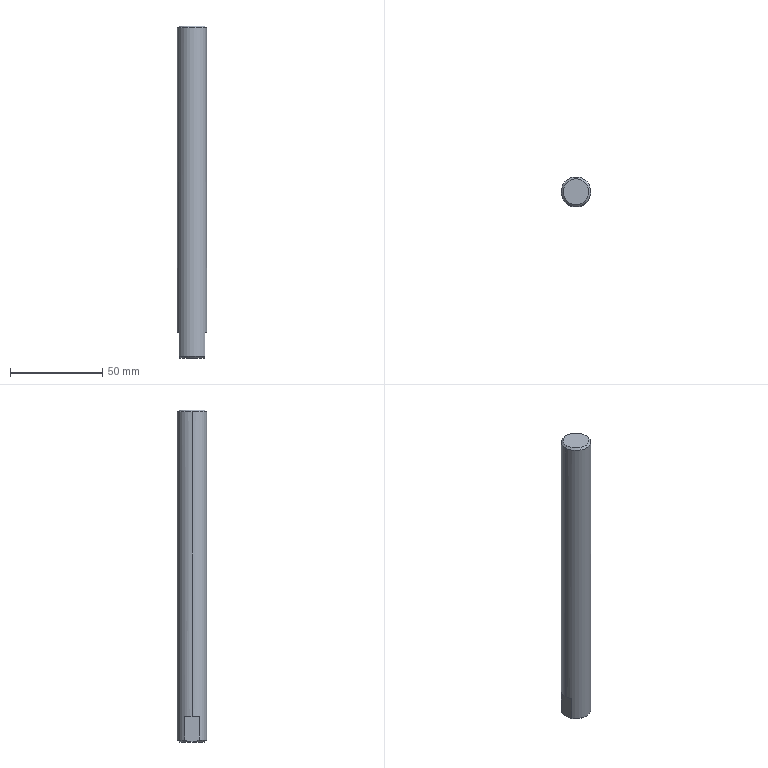Part | STEP file | PN_0110 Mount electronic clip adjusting screw rod | 1 solid | 12 faces | box 16 x 16 x 180 mm | volume 36003 mm3 | plane 6 | cone 4 | cylinder 2 | commonest cylinder face diameters 16 x2
STEP:
#1=CARTESIAN_POINT('',(0.,0.,0.));
#2=DIRECTION('',(0.,0.,1.));
#3=DIRECTION('',(1.,0.,0.));
#4=AXIS2_PLACEMENT_3D('',#1,#2,#3);
#5=CARTESIAN_POINT('',(7.,0.,180.));
#6=VERTEX_POINT('',#5);
#7=CARTESIAN_POINT('',(-7.,0.,180.));
#8=VERTEX_POINT('',#7);
#9=CARTESIAN_POINT('',(0.,0.,180.));
#10=DIRECTION('',(0.,0.,1.));
#11=DIRECTION('',(1.,0.,0.));
#12=AXIS2_PLACEMENT_3D('',#9,#10,#11);
#13=CIRCLE('',#12,7.);
#14=CARTESIAN_POINT('',(0.,0.,180.));
#15=DIRECTION('',(0.,0.,-1.));
#16=DIRECTION('',(-1.,0.,0.));
#17=AXIS2_PLACEMENT_3D('',#14,#15,#16);
#18=CONICAL_SURFACE('',#17,7.,0.7854);
#19=CARTESIAN_POINT('',(3.142,0.));
#20=DIRECTION('',(-1.,0.));
#21=VECTOR('',#20,1.);
#22=LINE('',#19,#21);
#23=(GEOMETRIC_REPRESENTATION_CONTEXT(2)PARAMETRIC_REPRESENTATION_CONTEXT()REPRESENTATION_CONTEXT('',''));
#24=DEFINITIONAL_REPRESENTATION('',(#22),#23);
#25=PCURVE('',#18,#24);
#26=CARTESIAN_POINT('',(0.,0.,180.));
#27=DIRECTION('',(0.,0.,1.));
#28=DIRECTION('',(1.,0.,0.));
#29=AXIS2_PLACEMENT_3D('',#26,#27,#28);
#30=PLANE('',#29);
#31=CARTESIAN_POINT('',(0.,0.));
#32=DIRECTION('',(1.,0.));
#33=AXIS2_PLACEMENT_2D('',#31,#32);
#34=CIRCLE('',#33,7.);
#35=(GEOMETRIC_REPRESENTATION_CONTEXT(2)PARAMETRIC_REPRESENTATION_CONTEXT()REPRESENTATION_CONTEXT('',''));
#36=DEFINITIONAL_REPRESENTATION('',(#34),#35);
#37=PCURVE('',#30,#36);
#38=SURFACE_CURVE('',#13,(#25,#37),.PCURVE_S1.);
#39=EDGE_CURVE('',#6,#8,#38,.T.);
#40=ORIENTED_EDGE('',*,*,#39,.F.);
#41=CARTESIAN_POINT('',(8.,0.,179.));
#42=VERTEX_POINT('',#41);
#43=CARTESIAN_POINT('',(7.,0.,180.));
#44=DIRECTION('',(0.7071,0.,-0.7071));
#45=VECTOR('',#44,1.);
#46=LINE('',#43,#45);
#47=CARTESIAN_POINT('',(3.142,0.));
#48=DIRECTION('',(0.,1.));
#49=VECTOR('',#48,1.);
#50=LINE('',#47,#49);
#51=(GEOMETRIC_REPRESENTATION_CONTEXT(2)PARAMETRIC_REPRESENTATION_CONTEXT()REPRESENTATION_CONTEXT('',''));
#52=DEFINITIONAL_REPRESENTATION('',(#50),#51);
#53=PCURVE('',#18,#52);
#54=CARTESIAN_POINT('',(0.,0.,180.));
#55=DIRECTION('',(0.,0.,-1.));
#56=DIRECTION('',(-1.,0.,0.));
#57=AXIS2_PLACEMENT_3D('',#54,#55,#56);
#58=CONICAL_SURFACE('',#57,7.,0.7854);
#59=CARTESIAN_POINT('',(3.142,0.));
#60=DIRECTION('',(0.,1.));
#61=VECTOR('',#60,1.);
#62=LINE('',#59,#61);
#63=(GEOMETRIC_REPRESENTATION_CONTEXT(2)PARAMETRIC_REPRESENTATION_CONTEXT()REPRESENTATION_CONTEXT('',''));
#64=DEFINITIONAL_REPRESENTATION('',(#62),#63);
#65=PCURVE('',#58,#64);
#66=SURFACE_CURVE('',#46,(#53,#65),.PCURVE_S1.);
#67=EDGE_CURVE('',#6,#42,#66,.T.);
#68=ORIENTED_EDGE('',*,*,#67,.T.);
#69=CARTESIAN_POINT('',(-8.,0.,179.));
#70=VERTEX_POINT('',#69);
#71=CARTESIAN_POINT('',(0.,0.,179.));
#72=DIRECTION('',(0.,0.,-1.));
#73=DIRECTION('',(1.,0.,0.));
#74=AXIS2_PLACEMENT_3D('',#71,#72,#73);
#75=CIRCLE('',#74,8.);
#76=CARTESIAN_POINT('',(-3.142,1.));
#77=DIRECTION('',(1.,0.));
#78=VECTOR('',#77,1.);
#79=LINE('',#76,#78);
#80=(GEOMETRIC_REPRESENTATION_CONTEXT(2)PARAMETRIC_REPRESENTATION_CONTEXT()REPRESENTATION_CONTEXT('',''));
#81=DEFINITIONAL_REPRESENTATION('',(#79),#80);
#82=PCURVE('',#18,#81);
#83=CARTESIAN_POINT('',(0.,0.,180.));
#84=DIRECTION('',(0.,0.,-1.));
#85=DIRECTION('',(-1.,0.,0.));
#86=AXIS2_PLACEMENT_3D('',#83,#84,#85);
#87=CYLINDRICAL_SURFACE('',#86,8.);
#88=CARTESIAN_POINT('',(-3.142,1.));
#89=DIRECTION('',(1.,0.));
#90=VECTOR('',#89,1.);
#91=LINE('',#88,#90);
#92=(GEOMETRIC_REPRESENTATION_CONTEXT(2)PARAMETRIC_REPRESENTATION_CONTEXT()REPRESENTATION_CONTEXT('',''));
#93=DEFINITIONAL_REPRESENTATION('',(#91),#92);
#94=PCURVE('',#87,#93);
#95=SURFACE_CURVE('',#75,(#82,#94),.PCURVE_S1.);
#96=EDGE_CURVE('',#70,#42,#95,.T.);
#97=ORIENTED_EDGE('',*,*,#96,.F.);
#98=CARTESIAN_POINT('',(-7.,0.,180.));
#99=DIRECTION('',(-0.7071,0.,-0.7071));
#100=VECTOR('',#99,1.);
#101=LINE('',#98,#100);
#102=CARTESIAN_POINT('',(0.,0.));
#103=DIRECTION('',(0.,1.));
#104=VECTOR('',#103,1.);
#105=LINE('',#102,#104);
#106=(GEOMETRIC_REPRESENTATION_CONTEXT(2)PARAMETRIC_REPRESENTATION_CONTEXT()REPRESENTATION_CONTEXT('',''));
#107=DEFINITIONAL_REPRESENTATION('',(#105),#106);
#108=PCURVE('',#18,#107);
#109=CARTESIAN_POINT('',(6.283,0.));
#110=DIRECTION('',(0.,1.));
#111=VECTOR('',#110,1.);
#112=LINE('',#109,#111);
#113=(GEOMETRIC_REPRESENTATION_CONTEXT(2)PARAMETRIC_REPRESENTATION_CONTEXT()REPRESENTATION_CONTEXT('',''));
#114=DEFINITIONAL_REPRESENTATION('',(#112),#113);
#115=PCURVE('',#58,#114);
#116=SURFACE_CURVE('',#101,(#108,#115),.PCURVE_S1.);
#117=EDGE_CURVE('',#8,#70,#116,.T.);
#118=ORIENTED_EDGE('',*,*,#117,.F.);
#119=EDGE_LOOP('',(#40,#68,#97,#118));
#120=FACE_BOUND('',#119,.T.);
#121=ADVANCED_FACE('',(#120),#18,.T.);
#122=ORIENTED_EDGE('',*,*,#96,.T.);
#123=CARTESIAN_POINT('',(8.,0.,14.));
#124=VERTEX_POINT('',#123);
#125=CARTESIAN_POINT('',(8.,0.,180.));
#126=DIRECTION('',(0.,0.,-1.));
#127=VECTOR('',#126,1.);
#128=LINE('',#125,#127);
#129=CARTESIAN_POINT('',(3.142,0.));
#130=DIRECTION('',(0.,1.));
#131=VECTOR('',#130,1.);
#132=LINE('',#129,#131);
#133=(GEOMETRIC_REPRESENTATION_CONTEXT(2)PARAMETRIC_REPRESENTATION_CONTEXT()REPRESENTATION_CONTEXT('',''));
#134=DEFINITIONAL_REPRESENTATION('',(#132),#133);
#135=PCURVE('',#87,#134);
#136=CARTESIAN_POINT('',(0.,0.,180.));
#137=DIRECTION('',(0.,0.,-1.));
#138=DIRECTION('',(-1.,0.,0.));
#139=AXIS2_PLACEMENT_3D('',#136,#137,#138);
#140=CYLINDRICAL_SURFACE('',#139,8.);
#141=CARTESIAN_POINT('',(3.142,0.));
#142=DIRECTION('',(0.,1.));
#143=VECTOR('',#142,1.);
#144=LINE('',#141,#143);
#145=(GEOMETRIC_REPRESENTATION_CONTEXT(2)PARAMETRIC_REPRESENTATION_CONTEXT()REPRESENTATION_CONTEXT('',''));
#146=DEFINITIONAL_REPRESENTATION('',(#144),#145);
#147=PCURVE('',#140,#146);
#148=SURFACE_CURVE('',#128,(#135,#147),.PCURVE_S1.);
#149=EDGE_CURVE('',#42,#124,#148,.T.);
#150=ORIENTED_EDGE('',*,*,#149,.T.);
#151=CARTESIAN_POINT('',(7.,3.873,14.));
#152=VERTEX_POINT('',#151);
#153=CARTESIAN_POINT('',(0.,0.,14.));
#154=DIRECTION('',(0.,0.,-1.));
#155=DIRECTION('',(-1.,0.,0.));
#156=AXIS2_PLACEMENT_3D('',#153,#154,#155);
#157=CIRCLE('',#156,8.);
#158=CARTESIAN_POINT('',(0.,166.));
#159=DIRECTION('',(1.,0.));
#160=VECTOR('',#159,1.);
#161=LINE('',#158,#160);
#162=(GEOMETRIC_REPRESENTATION_CONTEXT(2)PARAMETRIC_REPRESENTATION_CONTEXT()REPRESENTATION_CONTEXT('',''));
#163=DEFINITIONAL_REPRESENTATION('',(#161),#162);
#164=PCURVE('',#87,#163);
#165=CARTESIAN_POINT('',(0.,0.,14.));
#166=DIRECTION('',(0.,0.,-1.));
#167=DIRECTION('',(-1.,0.,0.));
#168=AXIS2_PLACEMENT_3D('',#165,#166,#167);
#169=PLANE('',#168);
#170=CARTESIAN_POINT('',(0.,0.));
#171=DIRECTION('',(1.,0.));
#172=AXIS2_PLACEMENT_2D('',#170,#171);
#173=CIRCLE('',#172,8.);
#174=(GEOMETRIC_REPRESENTATION_CONTEXT(2)PARAMETRIC_REPRESENTATION_CONTEXT()REPRESENTATION_CONTEXT('',''));
#175=DEFINITIONAL_REPRESENTATION('',(#173),#174);
#176=PCURVE('',#169,#175);
#177=SURFACE_CURVE('',#157,(#164,#176),.PCURVE_S1.);
#178=EDGE_CURVE('',#152,#124,#177,.T.);
#179=ORIENTED_EDGE('',*,*,#178,.F.);
#180=CARTESIAN_POINT('',(7.,3.873,1.));
#181=VERTEX_POINT('',#180);
#182=CARTESIAN_POINT('',(7.,3.873,180.));
#183=DIRECTION('',(0.,0.,-1.));
#184=VECTOR('',#183,1.);
#185=LINE('',#182,#184);
#186=CARTESIAN_POINT('',(2.636,0.));
#187=DIRECTION('',(0.,1.));
#188=VECTOR('',#187,1.);
#189=LINE('',#186,#188);
#190=(GEOMETRIC_REPRESENTATION_CONTEXT(2)PARAMETRIC_REPRESENTATION_CONTEXT()REPRESENTATION_CONTEXT('',''));
#191=DEFINITIONAL_REPRESENTATION('',(#189),#190);
#192=PCURVE('',#87,#191);
#193=CARTESIAN_POINT('',(7.,9.943,14.));
#194=DIRECTION('',(-1.,0.,0.));
#195=DIRECTION('',(0.,-1.,0.));
#196=AXIS2_PLACEMENT_3D('',#193,#194,#195);
#197=PLANE('',#196);
#198=CARTESIAN_POINT('',(6.07,166.));
#199=DIRECTION('',(0.,-1.));
#200=VECTOR('',#199,1.);
#201=LINE('',#198,#200);
#202=(GEOMETRIC_REPRESENTATION_CONTEXT(2)PARAMETRIC_REPRESENTATION_CONTEXT()REPRESENTATION_CONTEXT('',''));
#203=DEFINITIONAL_REPRESENTATION('',(#201),#202);
#204=PCURVE('',#197,#203);
#205=SURFACE_CURVE('',#185,(#192,#204),.PCURVE_S1.);
#206=EDGE_CURVE('',#152,#181,#205,.T.);
#207=ORIENTED_EDGE('',*,*,#206,.T.);
#208=CARTESIAN_POINT('',(-7.,3.873,1.));
#209=VERTEX_POINT('',#208);
#210=CARTESIAN_POINT('',(0.,0.,1.));
#211=DIRECTION('',(0.,0.,1.));
#212=DIRECTION('',(1.,0.,0.));
#213=AXIS2_PLACEMENT_3D('',#210,#211,#212);
#214=CIRCLE('',#213,8.);
#215=CARTESIAN_POINT('',(3.142,179.));
#216=DIRECTION('',(-1.,0.));
#217=VECTOR('',#216,1.);
#218=LINE('',#215,#217);
#219=(GEOMETRIC_REPRESENTATION_CONTEXT(2)PARAMETRIC_REPRESENTATION_CONTEXT()REPRESENTATION_CONTEXT('',''));
#220=DEFINITIONAL_REPRESENTATION('',(#218),#219);
#221=PCURVE('',#87,#220);
#222=CARTESIAN_POINT('',(0.,0.,1.));
#223=DIRECTION('',(0.,0.,1.));
#224=DIRECTION('',(1.,0.,0.));
#225=AXIS2_PLACEMENT_3D('',#222,#223,#224);
#226=CONICAL_SURFACE('',#225,8.,0.7854);
#227=CARTESIAN_POINT('',(0.,0.));
#228=DIRECTION('',(1.,0.));
#229=VECTOR('',#228,1.);
#230=LINE('',#227,#229);
#231=(GEOMETRIC_REPRESENTATION_CONTEXT(2)PARAMETRIC_REPRESENTATION_CONTEXT()REPRESENTATION_CONTEXT('',''));
#232=DEFINITIONAL_REPRESENTATION('',(#230),#231);
#233=PCURVE('',#226,#232);
#234=SURFACE_CURVE('',#214,(#221,#233),.PCURVE_S1.);
#235=EDGE_CURVE('',#181,#209,#234,.T.);
#236=ORIENTED_EDGE('',*,*,#235,.T.);
#237=CARTESIAN_POINT('',(-7.,3.873,14.));
#238=VERTEX_POINT('',#237);
#239=CARTESIAN_POINT('',(-7.,3.873,180.));
#240=DIRECTION('',(0.,0.,1.));
#241=VECTOR('',#240,1.);
#242=LINE('',#239,#241);
#243=CARTESIAN_POINT('',(0.5054,0.));
#244=DIRECTION('',(0.,-1.));
#245=VECTOR('',#244,1.);
#246=LINE('',#243,#245);
#247=(GEOMETRIC_REPRESENTATION_CONTEXT(2)PARAMETRIC_REPRESENTATION_CONTEXT()REPRESENTATION_CONTEXT('',''));
#248=DEFINITIONAL_REPRESENTATION('',(#246),#247);
#249=PCURVE('',#87,#248);
#250=CARTESIAN_POINT('',(-7.,9.943,14.));
#251=DIRECTION('',(1.,0.,0.));
#252=DIRECTION('',(0.,1.,0.));
#253=AXIS2_PLACEMENT_3D('',#250,#251,#252);
#254=PLANE('',#253);
#255=CARTESIAN_POINT('',(-6.07,166.));
#256=DIRECTION('',(0.,1.));
#257=VECTOR('',#256,1.);
#258=LINE('',#255,#257);
#259=(GEOMETRIC_REPRESENTATION_CONTEXT(2)PARAMETRIC_REPRESENTATION_CONTEXT()REPRESENTATION_CONTEXT('',''));
#260=DEFINITIONAL_REPRESENTATION('',(#258),#259);
#261=PCURVE('',#254,#260);
#262=SURFACE_CURVE('',#242,(#249,#261),.PCURVE_S1.);
#263=EDGE_CURVE('',#209,#238,#262,.T.);
#264=ORIENTED_EDGE('',*,*,#263,.T.);
#265=CARTESIAN_POINT('',(-8.,0.,14.));
#266=VERTEX_POINT('',#265);
#267=CARTESIAN_POINT('',(0.,0.,14.));
#268=DIRECTION('',(0.,0.,1.));
#269=DIRECTION('',(1.,0.,0.));
#270=AXIS2_PLACEMENT_3D('',#267,#268,#269);
#271=CIRCLE('',#270,8.);
#272=CARTESIAN_POINT('',(3.142,166.));
#273=DIRECTION('',(-1.,0.));
#274=VECTOR('',#273,1.);
#275=LINE('',#272,#274);
#276=(GEOMETRIC_REPRESENTATION_CONTEXT(2)PARAMETRIC_REPRESENTATION_CONTEXT()REPRESENTATION_CONTEXT('',''));
#277=DEFINITIONAL_REPRESENTATION('',(#275),#276);
#278=PCURVE('',#87,#277);
#279=CARTESIAN_POINT('',(0.,0.,14.));
#280=DIRECTION('',(0.,0.,1.));
#281=DIRECTION('',(1.,0.,0.));
#282=AXIS2_PLACEMENT_3D('',#279,#280,#281);
#283=PLANE('',#282);
#284=CARTESIAN_POINT('',(0.,0.));
#285=DIRECTION('',(1.,0.));
#286=AXIS2_PLACEMENT_2D('',#284,#285);
#287=CIRCLE('',#286,8.);
#288=(GEOMETRIC_REPRESENTATION_CONTEXT(2)PARAMETRIC_REPRESENTATION_CONTEXT()REPRESENTATION_CONTEXT('',''));
#289=DEFINITIONAL_REPRESENTATION('',(#287),#288);
#290=PCURVE('',#283,#289);
#291=SURFACE_CURVE('',#271,(#278,#290),.PCURVE_S1.);
#292=EDGE_CURVE('',#238,#266,#291,.T.);
#293=ORIENTED_EDGE('',*,*,#292,.T.);
#294=CARTESIAN_POINT('',(-8.,0.,180.));
#295=DIRECTION('',(0.,0.,-1.));
#296=VECTOR('',#295,1.);
#297=LINE('',#294,#296);
#298=CARTESIAN_POINT('',(0.,0.));
#299=DIRECTION('',(0.,1.));
#300=VECTOR('',#299,1.);
#301=LINE('',#298,#300);
#302=(GEOMETRIC_REPRESENTATION_CONTEXT(2)PARAMETRIC_REPRESENTATION_CONTEXT()REPRESENTATION_CONTEXT('',''));
#303=DEFINITIONAL_REPRESENTATION('',(#301),#302);
#304=PCURVE('',#87,#303);
#305=CARTESIAN_POINT('',(6.283,0.));
#306=DIRECTION('',(0.,1.));
#307=VECTOR('',#306,1.);
#308=LINE('',#305,#307);
#309=(GEOMETRIC_REPRESENTATION_CONTEXT(2)PARAMETRIC_REPRESENTATION_CONTEXT()REPRESENTATION_CONTEXT('',''));
#310=DEFINITIONAL_REPRESENTATION('',(#308),#309);
#311=PCURVE('',#140,#310);
#312=SURFACE_CURVE('',#297,(#304,#311),.PCURVE_S1.);
#313=EDGE_CURVE('',#70,#266,#312,.T.);
#314=ORIENTED_EDGE('',*,*,#313,.F.);
#315=EDGE_LOOP('',(#122,#150,#179,#207,#236,#264,#293,#314));
#316=FACE_BOUND('',#315,.T.);
#317=ADVANCED_FACE('',(#316),#87,.T.);
#318=ORIENTED_EDGE('',*,*,#149,.F.);
#319=CARTESIAN_POINT('',(0.,0.,179.));
#320=DIRECTION('',(0.,0.,-1.));
#321=DIRECTION('',(1.,0.,0.));
#322=AXIS2_PLACEMENT_3D('',#319,#320,#321);
#323=CIRCLE('',#322,8.);
#324=CARTESIAN_POINT('',(3.142,1.));
#325=DIRECTION('',(1.,0.));
#326=VECTOR('',#325,1.);
#327=LINE('',#324,#326);
#328=(GEOMETRIC_REPRESENTATION_CONTEXT(2)PARAMETRIC_REPRESENTATION_CONTEXT()REPRESENTATION_CONTEXT('',''));
#329=DEFINITIONAL_REPRESENTATION('',(#327),#328);
#330=PCURVE('',#140,#329);
#331=CARTESIAN_POINT('',(3.142,1.));
#332=DIRECTION('',(1.,0.));
#333=VECTOR('',#332,1.);
#334=LINE('',#331,#333);
#335=(GEOMETRIC_REPRESENTATION_CONTEXT(2)PARAMETRIC_REPRESENTATION_CONTEXT()REPRESENTATION_CONTEXT('',''));
#336=DEFINITIONAL_REPRESENTATION('',(#334),#335);
#337=PCURVE('',#58,#336);
#338=SURFACE_CURVE('',#323,(#330,#337),.PCURVE_S1.);
#339=EDGE_CURVE('',#42,#70,#338,.T.);
#340=ORIENTED_EDGE('',*,*,#339,.T.);
#341=ORIENTED_EDGE('',*,*,#313,.T.);
#342=CARTESIAN_POINT('',(-7.,-3.873,14.));
#343=VERTEX_POINT('',#342);
#344=CARTESIAN_POINT('',(0.,0.,14.));
#345=DIRECTION('',(0.,0.,1.));
#346=DIRECTION('',(1.,0.,0.));
#347=AXIS2_PLACEMENT_3D('',#344,#345,#346);
#348=CIRCLE('',#347,8.);
#349=CARTESIAN_POINT('',(9.425,166.));
#350=DIRECTION('',(-1.,0.));
#351=VECTOR('',#350,1.);
#352=LINE('',#349,#351);
#353=(GEOMETRIC_REPRESENTATION_CONTEXT(2)PARAMETRIC_REPRESENTATION_CONTEXT()REPRESENTATION_CONTEXT('',''));
#354=DEFINITIONAL_REPRESENTATION('',(#352),#353);
#355=PCURVE('',#140,#354);
#356=CARTESIAN_POINT('',(0.,0.));
#357=DIRECTION('',(1.,0.));
#358=AXIS2_PLACEMENT_2D('',#356,#357);
#359=CIRCLE('',#358,8.);
#360=(GEOMETRIC_REPRESENTATION_CONTEXT(2)PARAMETRIC_REPRESENTATION_CONTEXT()REPRESENTATION_CONTEXT('',''));
#361=DEFINITIONAL_REPRESENTATION('',(#359),#360);
#362=PCURVE('',#283,#361);
#363=SURFACE_CURVE('',#348,(#355,#362),.PCURVE_S1.);
#364=EDGE_CURVE('',#266,#343,#363,.T.);
#365=ORIENTED_EDGE('',*,*,#364,.T.);
#366=CARTESIAN_POINT('',(-7.,-3.873,1.));
#367=VERTEX_POINT('',#366);
#368=CARTESIAN_POINT('',(-7.,-3.873,180.));
#369=DIRECTION('',(0.,0.,-1.));
#370=VECTOR('',#369,1.);
#371=LINE('',#368,#370);
#372=CARTESIAN_POINT('',(5.778,0.));
#373=DIRECTION('',(0.,1.));
#374=VECTOR('',#373,1.);
#375=LINE('',#372,#374);
#376=(GEOMETRIC_REPRESENTATION_CONTEXT(2)PARAMETRIC_REPRESENTATION_CONTEXT()REPRESENTATION_CONTEXT('',''));
#377=DEFINITIONAL_REPRESENTATION('',(#375),#376);
#378=PCURVE('',#140,#377);
#379=CARTESIAN_POINT('',(-13.816,166.));
#380=DIRECTION('',(0.,-1.));
#381=VECTOR('',#380,1.);
#382=LINE('',#379,#381);
#383=(GEOMETRIC_REPRESENTATION_CONTEXT(2)PARAMETRIC_REPRESENTATION_CONTEXT()REPRESENTATION_CONTEXT('',''));
#384=DEFINITIONAL_REPRESENTATION('',(#382),#383);
#385=PCURVE('',#254,#384);
#386=SURFACE_CURVE('',#371,(#378,#385),.PCURVE_S1.);
#387=EDGE_CURVE('',#343,#367,#386,.T.);
#388=ORIENTED_EDGE('',*,*,#387,.T.);
#389=CARTESIAN_POINT('',(7.,-3.873,1.));
#390=VERTEX_POINT('',#389);
#391=CARTESIAN_POINT('',(0.,0.,1.));
#392=DIRECTION('',(0.,0.,1.));
#393=DIRECTION('',(1.,0.,0.));
#394=AXIS2_PLACEMENT_3D('',#391,#392,#393);
#395=CIRCLE('',#394,8.);
#396=CARTESIAN_POINT('',(9.425,179.));
#397=DIRECTION('',(-1.,0.));
#398=VECTOR('',#397,1.);
#399=LINE('',#396,#398);
#400=(GEOMETRIC_REPRESENTATION_CONTEXT(2)PARAMETRIC_REPRESENTATION_CONTEXT()REPRESENTATION_CONTEXT('',''));
#401=DEFINITIONAL_REPRESENTATION('',(#399),#400);
#402=PCURVE('',#140,#401);
#403=CARTESIAN_POINT('',(0.,0.,1.));
#404=DIRECTION('',(0.,0.,1.));
#405=DIRECTION('',(1.,0.,0.));
#406=AXIS2_PLACEMENT_3D('',#403,#404,#405);
#407=CONICAL_SURFACE('',#406,8.,0.7854);
#408=CARTESIAN_POINT('',(0.,0.));
#409=DIRECTION('',(1.,0.));
#410=VECTOR('',#409,1.);
#411=LINE('',#408,#410);
#412=(GEOMETRIC_REPRESENTATION_CONTEXT(2)PARAMETRIC_REPRESENTATION_CONTEXT()REPRESENTATION_CONTEXT('',''));
#413=DEFINITIONAL_REPRESENTATION('',(#411),#412);
#414=PCURVE('',#407,#413);
#415=SURFACE_CURVE('',#395,(#402,#414),.PCURVE_S1.);
#416=EDGE_CURVE('',#367,#390,#415,.T.);
#417=ORIENTED_EDGE('',*,*,#416,.T.);
#418=CARTESIAN_POINT('',(7.,-3.873,14.));
#419=VERTEX_POINT('',#418);
#420=CARTESIAN_POINT('',(7.,-3.873,180.));
#421=DIRECTION('',(0.,0.,1.));
#422=VECTOR('',#421,1.);
#423=LINE('',#420,#422);
#424=CARTESIAN_POINT('',(3.647,0.));
#425=DIRECTION('',(0.,-1.));
#426=VECTOR('',#425,1.);
#427=LINE('',#424,#426);
#428=(GEOMETRIC_REPRESENTATION_CONTEXT(2)PARAMETRIC_REPRESENTATION_CONTEXT()REPRESENTATION_CONTEXT('',''));
#429=DEFINITIONAL_REPRESENTATION('',(#427),#428);
#430=PCURVE('',#140,#429);
#431=CARTESIAN_POINT('',(13.816,166.));
#432=DIRECTION('',(0.,1.));
#433=VECTOR('',#432,1.);
#434=LINE('',#431,#433);
#435=(GEOMETRIC_REPRESENTATION_CONTEXT(2)PARAMETRIC_REPRESENTATION_CONTEXT()REPRESENTATION_CONTEXT('',''));
#436=DEFINITIONAL_REPRESENTATION('',(#434),#435);
#437=PCURVE('',#197,#436);
#438=SURFACE_CURVE('',#423,(#430,#437),.PCURVE_S1.);
#439=EDGE_CURVE('',#390,#419,#438,.T.);
#440=ORIENTED_EDGE('',*,*,#439,.T.);
#441=CARTESIAN_POINT('',(0.,0.,14.));
#442=DIRECTION('',(0.,0.,-1.));
#443=DIRECTION('',(-1.,0.,0.));
#444=AXIS2_PLACEMENT_3D('',#441,#442,#443);
#445=CIRCLE('',#444,8.);
#446=CARTESIAN_POINT('',(0.,166.));
#447=DIRECTION('',(1.,0.));
#448=VECTOR('',#447,1.);
#449=LINE('',#446,#448);
#450=(GEOMETRIC_REPRESENTATION_CONTEXT(2)PARAMETRIC_REPRESENTATION_CONTEXT()REPRESENTATION_CONTEXT('',''));
#451=DEFINITIONAL_REPRESENTATION('',(#449),#450);
#452=PCURVE('',#140,#451);
#453=CARTESIAN_POINT('',(0.,0.));
#454=DIRECTION('',(1.,0.));
#455=AXIS2_PLACEMENT_2D('',#453,#454);
#456=CIRCLE('',#455,8.);
#457=(GEOMETRIC_REPRESENTATION_CONTEXT(2)PARAMETRIC_REPRESENTATION_CONTEXT()REPRESENTATION_CONTEXT('',''));
#458=DEFINITIONAL_REPRESENTATION('',(#456),#457);
#459=PCURVE('',#169,#458);
#460=SURFACE_CURVE('',#445,(#452,#459),.PCURVE_S1.);
#461=EDGE_CURVE('',#124,#419,#460,.T.);
#462=ORIENTED_EDGE('',*,*,#461,.F.);
#463=EDGE_LOOP('',(#318,#340,#341,#365,#388,#417,#440,#462));
#464=FACE_BOUND('',#463,.T.);
#465=ADVANCED_FACE('',(#464),#140,.T.);
#466=CARTESIAN_POINT('',(0.,0.,180.));
#467=DIRECTION('',(0.,0.,1.));
#468=DIRECTION('',(1.,0.,0.));
#469=AXIS2_PLACEMENT_3D('',#466,#467,#468);
#470=CIRCLE('',#469,7.);
#471=CARTESIAN_POINT('',(0.,0.));
#472=DIRECTION('',(1.,0.));
#473=AXIS2_PLACEMENT_2D('',#471,#472);
#474=CIRCLE('',#473,7.);
#475=(GEOMETRIC_REPRESENTATION_CONTEXT(2)PARAMETRIC_REPRESENTATION_CONTEXT()REPRESENTATION_CONTEXT('',''));
#476=DEFINITIONAL_REPRESENTATION('',(#474),#475);
#477=PCURVE('',#30,#476);
#478=CARTESIAN_POINT('',(9.425,0.));
#479=DIRECTION('',(-1.,0.));
#480=VECTOR('',#479,1.);
#481=LINE('',#478,#480);
#482=(GEOMETRIC_REPRESENTATION_CONTEXT(2)PARAMETRIC_REPRESENTATION_CONTEXT()REPRESENTATION_CONTEXT('',''));
#483=DEFINITIONAL_REPRESENTATION('',(#481),#482);
#484=PCURVE('',#58,#483);
#485=SURFACE_CURVE('',#470,(#477,#484),.PCURVE_S1.);
#486=EDGE_CURVE('',#8,#6,#485,.T.);
#487=ORIENTED_EDGE('',*,*,#486,.T.);
#488=ORIENTED_EDGE('',*,*,#39,.T.);
#489=EDGE_LOOP('',(#487,#488));
#490=FACE_BOUND('',#489,.T.);
#491=ADVANCED_FACE('',(#490),#30,.T.);
#492=CARTESIAN_POINT('',(-7.,0.,0.));
#493=VERTEX_POINT('',#492);
#494=CARTESIAN_POINT('',(7.,0.,0.));
#495=VERTEX_POINT('',#494);
#496=CARTESIAN_POINT('',(0.,0.,0.));
#497=DIRECTION('',(0.,0.,-1.));
#498=DIRECTION('',(1.,0.,0.));
#499=AXIS2_PLACEMENT_3D('',#496,#497,#498);
#500=CIRCLE('',#499,7.);
#501=CARTESIAN_POINT('',(0.,0.,0.));
#502=DIRECTION('',(0.,0.,1.));
#503=DIRECTION('',(1.,0.,0.));
#504=AXIS2_PLACEMENT_3D('',#501,#502,#503);
#505=PLANE('',#504);
#506=CARTESIAN_POINT('',(7.,0.));
#507=CARTESIAN_POINT('',(7.,-12.124));
#508=CARTESIAN_POINT('',(-3.5,-6.062));
#509=CARTESIAN_POINT('',(-14.,0.));
#510=CARTESIAN_POINT('',(-3.5,6.062));
#511=CARTESIAN_POINT('',(7.,12.124));
#512=CARTESIAN_POINT('',(7.,0.));
#513=(BOUNDED_CURVE()B_SPLINE_CURVE(2,(#506,#507,#508,#509,#510,#511,#512),.UNSPECIFIED.,.T.,.F.)B_SPLINE_CURVE_WITH_KNOTS((1,2,2,2,2,1),(-2.094,0.,2.094,4.189,6.283,8.378),.UNSPECIFIED.)CURVE()GEOMETRIC_REPRESENTATION_ITEM()RATIONAL_B_SPLINE_CURVE((1.,0.5,1.,0.5,1.,0.5,1.))REPRESENTATION_ITEM(''));
#514=(GEOMETRIC_REPRESENTATION_CONTEXT(2)PARAMETRIC_REPRESENTATION_CONTEXT()REPRESENTATION_CONTEXT('',''));
#515=DEFINITIONAL_REPRESENTATION('',(#513),#514);
#516=PCURVE('',#505,#515);
#517=CARTESIAN_POINT('',(6.283,-1.));
#518=DIRECTION('',(-1.,0.));
#519=VECTOR('',#518,1.);
#520=LINE('',#517,#519);
#521=(GEOMETRIC_REPRESENTATION_CONTEXT(2)PARAMETRIC_REPRESENTATION_CONTEXT()REPRESENTATION_CONTEXT('',''));
#522=DEFINITIONAL_REPRESENTATION('',(#520),#521);
#523=PCURVE('',#226,#522);
#524=SURFACE_CURVE('',#500,(#516,#523),.PCURVE_S1.);
#525=EDGE_CURVE('',#493,#495,#524,.T.);
#526=ORIENTED_EDGE('',*,*,#525,.T.);
#527=CARTESIAN_POINT('',(0.,0.,0.));
#528=DIRECTION('',(0.,0.,-1.));
#529=DIRECTION('',(1.,0.,0.));
#530=AXIS2_PLACEMENT_3D('',#527,#528,#529);
#531=CIRCLE('',#530,7.);
#532=CARTESIAN_POINT('',(7.,0.));
#533=CARTESIAN_POINT('',(7.,-12.124));
#534=CARTESIAN_POINT('',(-3.5,-6.062));
#535=CARTESIAN_POINT('',(-14.,0.));
#536=CARTESIAN_POINT('',(-3.5,6.062));
#537=CARTESIAN_POINT('',(7.,12.124));
#538=CARTESIAN_POINT('',(7.,0.));
#539=(BOUNDED_CURVE()B_SPLINE_CURVE(2,(#532,#533,#534,#535,#536,#537,#538),.UNSPECIFIED.,.T.,.F.)B_SPLINE_CURVE_WITH_KNOTS((1,2,2,2,2,1),(-2.094,0.,2.094,4.189,6.283,8.378),.UNSPECIFIED.)CURVE()GEOMETRIC_REPRESENTATION_ITEM()RATIONAL_B_SPLINE_CURVE((1.,0.5,1.,0.5,1.,0.5,1.))REPRESENTATION_ITEM(''));
#540=(GEOMETRIC_REPRESENTATION_CONTEXT(2)PARAMETRIC_REPRESENTATION_CONTEXT()REPRESENTATION_CONTEXT('',''));
#541=DEFINITIONAL_REPRESENTATION('',(#539),#540);
#542=PCURVE('',#505,#541);
#543=CARTESIAN_POINT('',(6.283,-1.));
#544=DIRECTION('',(-1.,0.));
#545=VECTOR('',#544,1.);
#546=LINE('',#543,#545);
#547=(GEOMETRIC_REPRESENTATION_CONTEXT(2)PARAMETRIC_REPRESENTATION_CONTEXT()REPRESENTATION_CONTEXT('',''));
#548=DEFINITIONAL_REPRESENTATION('',(#546),#547);
#549=PCURVE('',#407,#548);
#550=SURFACE_CURVE('',#531,(#542,#549),.PCURVE_S1.);
#551=EDGE_CURVE('',#495,#493,#550,.T.);
#552=ORIENTED_EDGE('',*,*,#551,.T.);
#553=EDGE_LOOP('',(#526,#552));
#554=FACE_BOUND('',#553,.T.);
#555=ADVANCED_FACE('',(#554),#505,.F.);
#556=ORIENTED_EDGE('',*,*,#178,.T.);
#557=ORIENTED_EDGE('',*,*,#461,.T.);
#558=CARTESIAN_POINT('',(7.,9.943,14.));
#559=DIRECTION('',(0.,1.,0.));
#560=VECTOR('',#559,1.);
#561=LINE('',#558,#560);
#562=CARTESIAN_POINT('',(-7.,9.943));
#563=DIRECTION('',(0.,1.));
#564=VECTOR('',#563,1.);
#565=LINE('',#562,#564);
#566=(GEOMETRIC_REPRESENTATION_CONTEXT(2)PARAMETRIC_REPRESENTATION_CONTEXT()REPRESENTATION_CONTEXT('',''));
#567=DEFINITIONAL_REPRESENTATION('',(#565),#566);
#568=PCURVE('',#169,#567);
#569=CARTESIAN_POINT('',(0.,0.));
#570=DIRECTION('',(-1.,0.));
#571=VECTOR('',#570,1.);
#572=LINE('',#569,#571);
#573=(GEOMETRIC_REPRESENTATION_CONTEXT(2)PARAMETRIC_REPRESENTATION_CONTEXT()REPRESENTATION_CONTEXT('',''));
#574=DEFINITIONAL_REPRESENTATION('',(#572),#573);
#575=PCURVE('',#197,#574);
#576=SURFACE_CURVE('',#561,(#568,#575),.PCURVE_S1.);
#577=EDGE_CURVE('',#419,#152,#576,.T.);
#578=ORIENTED_EDGE('',*,*,#577,.T.);
#579=EDGE_LOOP('',(#556,#557,#578));
#580=FACE_BOUND('',#579,.T.);
#581=ADVANCED_FACE('',(#580),#169,.T.);
#582=ORIENTED_EDGE('',*,*,#439,.F.);
#583=CARTESIAN_POINT('',(7.,-3.873,1.));
#584=CARTESIAN_POINT('',(7.,-3.264,0.7051));
#585=CARTESIAN_POINT('',(7.,-2.642,0.4562));
#586=CARTESIAN_POINT('',(7.,-1.677,0.1913));
#587=CARTESIAN_POINT('',(7.,-1.35,0.1213));
#588=CARTESIAN_POINT('',(7.,-0.683,0.0255));
#589=CARTESIAN_POINT('',(7.,-0.3413,0.));
#590=CARTESIAN_POINT('',(7.,0.,0.));
#591=B_SPLINE_CURVE_WITH_KNOTS('',3,(#583,#584,#585,#586,#587,#588,#589,#590),.UNSPECIFIED.,.F.,.F.,(4,2,2,4),(0.,0.002001,0.003002,0.004002),.UNSPECIFIED.);
#592=CARTESIAN_POINT('',(13.816,-13.));
#593=CARTESIAN_POINT('',(13.207,-13.295));
#594=CARTESIAN_POINT('',(12.584,-13.544));
#595=CARTESIAN_POINT('',(11.619,-13.809));
#596=CARTESIAN_POINT('',(11.293,-13.879));
#597=CARTESIAN_POINT('',(10.626,-13.975));
#598=CARTESIAN_POINT('',(10.284,-14.));
#599=CARTESIAN_POINT('',(9.943,-14.));
#600=B_SPLINE_CURVE_WITH_KNOTS('',3,(#592,#593,#594,#595,#596,#597,#598,#599),.UNSPECIFIED.,.F.,.F.,(4,2,2,4),(0.,0.002001,0.003002,0.004002),.UNSPECIFIED.);
#601=(GEOMETRIC_REPRESENTATION_CONTEXT(2)PARAMETRIC_REPRESENTATION_CONTEXT()REPRESENTATION_CONTEXT('',''));
#602=DEFINITIONAL_REPRESENTATION('',(#600),#601);
#603=PCURVE('',#197,#602);
#604=CARTESIAN_POINT('',(5.778,0.));
#605=CARTESIAN_POINT('',(5.784,-0.02681));
#606=CARTESIAN_POINT('',(5.796,-0.07965));
#607=CARTESIAN_POINT('',(5.815,-0.1565));
#608=CARTESIAN_POINT('',(5.834,-0.2309));
#609=CARTESIAN_POINT('',(5.854,-0.3026));
#610=CARTESIAN_POINT('',(5.874,-0.3715));
#611=CARTESIAN_POINT('',(5.895,-0.4376));
#612=CARTESIAN_POINT('',(5.916,-0.5008));
#613=CARTESIAN_POINT('',(5.938,-0.5608));
#614=CARTESIAN_POINT('',(5.96,-0.6176));
#615=CARTESIAN_POINT('',(5.982,-0.671));
#616=CARTESIAN_POINT('',(6.005,-0.721));
#617=CARTESIAN_POINT('',(6.028,-0.7673));
#618=CARTESIAN_POINT('',(6.052,-0.8099));
#619=CARTESIAN_POINT('',(6.077,-0.8486));
#620=CARTESIAN_POINT('',(6.101,-0.8833));
#621=CARTESIAN_POINT('',(6.126,-0.9137));
#622=CARTESIAN_POINT('',(6.152,-0.9399));
#623=CARTESIAN_POINT('',(6.178,-0.9615));
#624=CARTESIAN_POINT('',(6.204,-0.9786));
#625=CARTESIAN_POINT('',(6.23,-0.9909));
#626=CARTESIAN_POINT('',(6.257,-0.9983));
#627=CARTESIAN_POINT('',(6.274,-1.));
#628=CARTESIAN_POINT('',(6.283,-1.));
#629=B_SPLINE_CURVE_WITH_KNOTS('',3,(#604,#605,#606,#607,#608,#609,#610,#611,#612,#613,#614,#615,#616,#617,#618,#619,#620,#621,#622,#623,#624,#625,#626,#627,#628),.UNSPECIFIED.,.F.,.F.,(4,1,1,1,1,1,1,1,1,1,1,1,1,1,1,1,1,1,1,1,1,1,4),(0.,0.0001819,0.0003638,0.0005458,0.0007277,0.0009096,0.001092,0.001273,0.001455,0.001637,0.001819,0.002001,0.002183,0.002365,0.002547,0.002729,0.002911,0.003093,0.003275,0.003456,0.003638,0.00382,0.004002),.QUASI_UNIFORM_KNOTS.);
#630=(GEOMETRIC_REPRESENTATION_CONTEXT(2)PARAMETRIC_REPRESENTATION_CONTEXT()REPRESENTATION_CONTEXT('',''));
#631=DEFINITIONAL_REPRESENTATION('',(#629),#630);
#632=PCURVE('',#407,#631);
#633=SURFACE_CURVE('',#591,(#603,#632),.PCURVE_S1.);
#634=EDGE_CURVE('',#390,#495,#633,.T.);
#635=ORIENTED_EDGE('',*,*,#634,.T.);
#636=CARTESIAN_POINT('',(7.,0.,0.));
#637=CARTESIAN_POINT('',(7.,0.6781,0.));
#638=CARTESIAN_POINT('',(7.,1.339,0.09963));
#639=CARTESIAN_POINT('',(7.,2.31,0.3647));
#640=CARTESIAN_POINT('',(7.,2.631,0.4726));
#641=CARTESIAN_POINT('',(7.,3.26,0.7166));
#642=CARTESIAN_POINT('',(7.,3.569,0.8528));
#643=CARTESIAN_POINT('',(7.,3.873,1.));
#644=B_SPLINE_CURVE_WITH_KNOTS('',3,(#636,#637,#638,#639,#640,#641,#642,#643),.UNSPECIFIED.,.F.,.F.,(4,2,2,4),(0.,0.002004,0.003006,0.004009),.UNSPECIFIED.);
#645=CARTESIAN_POINT('',(9.943,-14.));
#646=CARTESIAN_POINT('',(9.265,-14.));
#647=CARTESIAN_POINT('',(8.604,-13.9));
#648=CARTESIAN_POINT('',(7.633,-13.635));
#649=CARTESIAN_POINT('',(7.312,-13.527));
#650=CARTESIAN_POINT('',(6.683,-13.283));
#651=CARTESIAN_POINT('',(6.374,-13.147));
#652=CARTESIAN_POINT('',(6.07,-13.));
#653=B_SPLINE_CURVE_WITH_KNOTS('',3,(#645,#646,#647,#648,#649,#650,#651,#652),.UNSPECIFIED.,.F.,.F.,(4,2,2,4),(0.,0.002004,0.003006,0.004009),.UNSPECIFIED.);
#654=(GEOMETRIC_REPRESENTATION_CONTEXT(2)PARAMETRIC_REPRESENTATION_CONTEXT()REPRESENTATION_CONTEXT('',''));
#655=DEFINITIONAL_REPRESENTATION('',(#653),#654);
#656=PCURVE('',#197,#655);
#657=CARTESIAN_POINT('',(0.,-1.));
#658=CARTESIAN_POINT('',(0.008807,-1.));
#659=CARTESIAN_POINT('',(0.02638,-0.9984));
#660=CARTESIAN_POINT('',(0.05258,-0.9911));
#661=CARTESIAN_POINT('',(0.07859,-0.9791));
#662=CARTESIAN_POINT('',(0.1044,-0.9624));
#663=CARTESIAN_POINT('',(0.1299,-0.9412));
#664=CARTESIAN_POINT('',(0.1552,-0.9155));
#665=CARTESIAN_POINT('',(0.1802,-0.8856));
#666=CARTESIAN_POINT('',(0.2048,-0.8513));
#667=CARTESIAN_POINT('',(0.2291,-0.813));
#668=CARTESIAN_POINT('',(0.253,-0.7706));
#669=CARTESIAN_POINT('',(0.2765,-0.7243));
#670=CARTESIAN_POINT('',(0.2997,-0.6742));
#671=CARTESIAN_POINT('',(0.3225,-0.6204));
#672=CARTESIAN_POINT('',(0.3448,-0.5631));
#673=CARTESIAN_POINT('',(0.3666,-0.5025));
#674=CARTESIAN_POINT('',(0.3879,-0.4388));
#675=CARTESIAN_POINT('',(0.4088,-0.3723));
#676=CARTESIAN_POINT('',(0.4291,-0.3029));
#677=CARTESIAN_POINT('',(0.4489,-0.231));
#678=CARTESIAN_POINT('',(0.4682,-0.1565));
#679=CARTESIAN_POINT('',(0.4871,-0.07957));
#680=CARTESIAN_POINT('',(0.4993,-0.02677));
#681=CARTESIAN_POINT('',(0.5054,0.));
#682=B_SPLINE_CURVE_WITH_KNOTS('',3,(#657,#658,#659,#660,#661,#662,#663,#664,#665,#666,#667,#668,#669,#670,#671,#672,#673,#674,#675,#676,#677,#678,#679,#680,#681),.UNSPECIFIED.,.F.,.F.,(4,1,1,1,1,1,1,1,1,1,1,1,1,1,1,1,1,1,1,1,1,1,4),(0.,0.0001822,0.0003644,0.0005466,0.0007288,0.000911,0.001093,0.001275,0.001458,0.00164,0.001822,0.002004,0.002186,0.002369,0.002551,0.002733,0.002915,0.003097,0.00328,0.003462,0.003644,0.003826,0.004009),.QUASI_UNIFORM_KNOTS.);
#683=(GEOMETRIC_REPRESENTATION_CONTEXT(2)PARAMETRIC_REPRESENTATION_CONTEXT()REPRESENTATION_CONTEXT('',''));
#684=DEFINITIONAL_REPRESENTATION('',(#682),#683);
#685=PCURVE('',#226,#684);
#686=SURFACE_CURVE('',#644,(#656,#685),.PCURVE_S1.);
#687=EDGE_CURVE('',#495,#181,#686,.T.);
#688=ORIENTED_EDGE('',*,*,#687,.T.);
#689=ORIENTED_EDGE('',*,*,#206,.F.);
#690=ORIENTED_EDGE('',*,*,#577,.F.);
#691=EDGE_LOOP('',(#582,#635,#688,#689,#690));
#692=FACE_BOUND('',#691,.T.);
#693=ADVANCED_FACE('',(#692),#197,.F.);
#694=CARTESIAN_POINT('',(-7.,9.943,14.));
#695=DIRECTION('',(0.,-1.,0.));
#696=VECTOR('',#695,1.);
#697=LINE('',#694,#696);
#698=CARTESIAN_POINT('',(-7.,9.943));
#699=DIRECTION('',(0.,-1.));
#700=VECTOR('',#699,1.);
#701=LINE('',#698,#700);
#702=(GEOMETRIC_REPRESENTATION_CONTEXT(2)PARAMETRIC_REPRESENTATION_CONTEXT()REPRESENTATION_CONTEXT('',''));
#703=DEFINITIONAL_REPRESENTATION('',(#701),#702);
#704=PCURVE('',#283,#703);
#705=CARTESIAN_POINT('',(0.,0.));
#706=DIRECTION('',(-1.,0.));
#707=VECTOR('',#706,1.);
#708=LINE('',#705,#707);
#709=(GEOMETRIC_REPRESENTATION_CONTEXT(2)PARAMETRIC_REPRESENTATION_CONTEXT()REPRESENTATION_CONTEXT('',''));
#710=DEFINITIONAL_REPRESENTATION('',(#708),#709);
#711=PCURVE('',#254,#710);
#712=SURFACE_CURVE('',#697,(#704,#711),.PCURVE_S1.);
#713=EDGE_CURVE('',#238,#343,#712,.T.);
#714=ORIENTED_EDGE('',*,*,#713,.T.);
#715=ORIENTED_EDGE('',*,*,#364,.F.);
#716=ORIENTED_EDGE('',*,*,#292,.F.);
#717=EDGE_LOOP('',(#714,#715,#716));
#718=FACE_BOUND('',#717,.T.);
#719=ADVANCED_FACE('',(#718),#283,.F.);
#720=CARTESIAN_POINT('',(-7.,3.873,1.));
#721=CARTESIAN_POINT('',(-7.,3.264,0.7051));
#722=CARTESIAN_POINT('',(-7.,2.642,0.4562));
#723=CARTESIAN_POINT('',(-7.,1.677,0.1913));
#724=CARTESIAN_POINT('',(-7.,1.35,0.1213));
#725=CARTESIAN_POINT('',(-7.,0.683,0.0255));
#726=CARTESIAN_POINT('',(-7.,0.3413,0.));
#727=CARTESIAN_POINT('',(-7.,0.,0.));
#728=B_SPLINE_CURVE_WITH_KNOTS('',3,(#720,#721,#722,#723,#724,#725,#726,#727),.UNSPECIFIED.,.F.,.F.,(4,2,2,4),(0.,0.002001,0.003002,0.004002),.UNSPECIFIED.);
#729=CARTESIAN_POINT('',(-6.07,-13.));
#730=CARTESIAN_POINT('',(-6.679,-13.295));
#731=CARTESIAN_POINT('',(-7.301,-13.544));
#732=CARTESIAN_POINT('',(-8.266,-13.809));
#733=CARTESIAN_POINT('',(-8.593,-13.879));
#734=CARTESIAN_POINT('',(-9.26,-13.975));
#735=CARTESIAN_POINT('',(-9.602,-14.));
#736=CARTESIAN_POINT('',(-9.943,-14.));
#737=B_SPLINE_CURVE_WITH_KNOTS('',3,(#729,#730,#731,#732,#733,#734,#735,#736),.UNSPECIFIED.,.F.,.F.,(4,2,2,4),(0.,0.002001,0.003002,0.004002),.UNSPECIFIED.);
#738=(GEOMETRIC_REPRESENTATION_CONTEXT(2)PARAMETRIC_REPRESENTATION_CONTEXT()REPRESENTATION_CONTEXT('',''));
#739=DEFINITIONAL_REPRESENTATION('',(#737),#738);
#740=PCURVE('',#254,#739);
#741=CARTESIAN_POINT('',(2.636,0.));
#742=CARTESIAN_POINT('',(2.642,-0.02681));
#743=CARTESIAN_POINT('',(2.655,-0.07965));
#744=CARTESIAN_POINT('',(2.673,-0.1565));
#745=CARTESIAN_POINT('',(2.693,-0.2309));
#746=CARTESIAN_POINT('',(2.712,-0.3026));
#747=CARTESIAN_POINT('',(2.733,-0.3715));
#748=CARTESIAN_POINT('',(2.753,-0.4376));
#749=CARTESIAN_POINT('',(2.774,-0.5008));
#750=CARTESIAN_POINT('',(2.796,-0.5608));
#751=CARTESIAN_POINT('',(2.818,-0.6176));
#752=CARTESIAN_POINT('',(2.84,-0.671));
#753=CARTESIAN_POINT('',(2.863,-0.721));
#754=CARTESIAN_POINT('',(2.887,-0.7673));
#755=CARTESIAN_POINT('',(2.911,-0.8099));
#756=CARTESIAN_POINT('',(2.935,-0.8486));
#757=CARTESIAN_POINT('',(2.96,-0.8833));
#758=CARTESIAN_POINT('',(2.985,-0.9137));
#759=CARTESIAN_POINT('',(3.01,-0.9399));
#760=CARTESIAN_POINT('',(3.036,-0.9615));
#761=CARTESIAN_POINT('',(3.062,-0.9786));
#762=CARTESIAN_POINT('',(3.088,-0.9909));
#763=CARTESIAN_POINT('',(3.115,-0.9983));
#764=CARTESIAN_POINT('',(3.133,-1.));
#765=CARTESIAN_POINT('',(3.142,-1.));
#766=B_SPLINE_CURVE_WITH_KNOTS('',3,(#741,#742,#743,#744,#745,#746,#747,#748,#749,#750,#751,#752,#753,#754,#755,#756,#757,#758,#759,#760,#761,#762,#763,#764,#765),.UNSPECIFIED.,.F.,.F.,(4,1,1,1,1,1,1,1,1,1,1,1,1,1,1,1,1,1,1,1,1,1,4),(0.,0.0001819,0.0003638,0.0005458,0.0007277,0.0009096,0.001092,0.001273,0.001455,0.001637,0.001819,0.002001,0.002183,0.002365,0.002547,0.002729,0.002911,0.003093,0.003275,0.003456,0.003638,0.00382,0.004002),.QUASI_UNIFORM_KNOTS.);
#767=(GEOMETRIC_REPRESENTATION_CONTEXT(2)PARAMETRIC_REPRESENTATION_CONTEXT()REPRESENTATION_CONTEXT('',''));
#768=DEFINITIONAL_REPRESENTATION('',(#766),#767);
#769=PCURVE('',#226,#768);
#770=SURFACE_CURVE('',#728,(#740,#769),.PCURVE_S1.);
#771=EDGE_CURVE('',#209,#493,#770,.T.);
#772=ORIENTED_EDGE('',*,*,#771,.T.);
#773=CARTESIAN_POINT('',(-7.,0.,0.));
#774=CARTESIAN_POINT('',(-7.,-0.6781,0.));
#775=CARTESIAN_POINT('',(-7.,-1.339,0.09963));
#776=CARTESIAN_POINT('',(-7.,-2.31,0.3647));
#777=CARTESIAN_POINT('',(-7.,-2.631,0.4726));
#778=CARTESIAN_POINT('',(-7.,-3.26,0.7166));
#779=CARTESIAN_POINT('',(-7.,-3.569,0.8528));
#780=CARTESIAN_POINT('',(-7.,-3.873,1.));
#781=B_SPLINE_CURVE_WITH_KNOTS('',3,(#773,#774,#775,#776,#777,#778,#779,#780),.UNSPECIFIED.,.F.,.F.,(4,2,2,4),(0.,0.002004,0.003006,0.004009),.UNSPECIFIED.);
#782=CARTESIAN_POINT('',(-9.943,-14.));
#783=CARTESIAN_POINT('',(-10.621,-14.));
#784=CARTESIAN_POINT('',(-11.282,-13.9));
#785=CARTESIAN_POINT('',(-12.253,-13.635));
#786=CARTESIAN_POINT('',(-12.574,-13.527));
#787=CARTESIAN_POINT('',(-13.203,-13.283));
#788=CARTESIAN_POINT('',(-13.512,-13.147));
#789=CARTESIAN_POINT('',(-13.816,-13.));
#790=B_SPLINE_CURVE_WITH_KNOTS('',3,(#782,#783,#784,#785,#786,#787,#788,#789),.UNSPECIFIED.,.F.,.F.,(4,2,2,4),(0.,0.002004,0.003006,0.004009),.UNSPECIFIED.);
#791=(GEOMETRIC_REPRESENTATION_CONTEXT(2)PARAMETRIC_REPRESENTATION_CONTEXT()REPRESENTATION_CONTEXT('',''));
#792=DEFINITIONAL_REPRESENTATION('',(#790),#791);
#793=PCURVE('',#254,#792);
#794=CARTESIAN_POINT('',(3.142,-1.));
#795=CARTESIAN_POINT('',(3.15,-1.));
#796=CARTESIAN_POINT('',(3.168,-0.9984));
#797=CARTESIAN_POINT('',(3.194,-0.9911));
#798=CARTESIAN_POINT('',(3.22,-0.9791));
#799=CARTESIAN_POINT('',(3.246,-0.9624));
#800=CARTESIAN_POINT('',(3.272,-0.9412));
#801=CARTESIAN_POINT('',(3.297,-0.9155));
#802=CARTESIAN_POINT('',(3.322,-0.8856));
#803=CARTESIAN_POINT('',(3.346,-0.8513));
#804=CARTESIAN_POINT('',(3.371,-0.813));
#805=CARTESIAN_POINT('',(3.395,-0.7706));
#806=CARTESIAN_POINT('',(3.418,-0.7243));
#807=CARTESIAN_POINT('',(3.441,-0.6742));
#808=CARTESIAN_POINT('',(3.464,-0.6204));
#809=CARTESIAN_POINT('',(3.486,-0.5631));
#810=CARTESIAN_POINT('',(3.508,-0.5025));
#811=CARTESIAN_POINT('',(3.53,-0.4388));
#812=CARTESIAN_POINT('',(3.55,-0.3723));
#813=CARTESIAN_POINT('',(3.571,-0.3029));
#814=CARTESIAN_POINT('',(3.59,-0.231));
#815=CARTESIAN_POINT('',(3.61,-0.1565));
#816=CARTESIAN_POINT('',(3.629,-0.07957));
#817=CARTESIAN_POINT('',(3.641,-0.02677));
#818=CARTESIAN_POINT('',(3.647,0.));
#819=B_SPLINE_CURVE_WITH_KNOTS('',3,(#794,#795,#796,#797,#798,#799,#800,#801,#802,#803,#804,#805,#806,#807,#808,#809,#810,#811,#812,#813,#814,#815,#816,#817,#818),.UNSPECIFIED.,.F.,.F.,(4,1,1,1,1,1,1,1,1,1,1,1,1,1,1,1,1,1,1,1,1,1,4),(0.,0.0001822,0.0003644,0.0005466,0.0007288,0.000911,0.001093,0.001275,0.001458,0.00164,0.001822,0.002004,0.002186,0.002369,0.002551,0.002733,0.002915,0.003097,0.00328,0.003462,0.003644,0.003826,0.004009),.QUASI_UNIFORM_KNOTS.);
#820=(GEOMETRIC_REPRESENTATION_CONTEXT(2)PARAMETRIC_REPRESENTATION_CONTEXT()REPRESENTATION_CONTEXT('',''));
#821=DEFINITIONAL_REPRESENTATION('',(#819),#820);
#822=PCURVE('',#407,#821);
#823=SURFACE_CURVE('',#781,(#793,#822),.PCURVE_S1.);
#824=EDGE_CURVE('',#493,#367,#823,.T.);
#825=ORIENTED_EDGE('',*,*,#824,.T.);
#826=ORIENTED_EDGE('',*,*,#387,.F.);
#827=ORIENTED_EDGE('',*,*,#713,.F.);
#828=ORIENTED_EDGE('',*,*,#263,.F.);
#829=EDGE_LOOP('',(#772,#825,#826,#827,#828));
#830=FACE_BOUND('',#829,.T.);
#831=ADVANCED_FACE('',(#830),#254,.F.);
#832=ORIENTED_EDGE('',*,*,#824,.F.);
#833=ORIENTED_EDGE('',*,*,#551,.F.);
#834=ORIENTED_EDGE('',*,*,#634,.F.);
#835=ORIENTED_EDGE('',*,*,#416,.F.);
#836=EDGE_LOOP('',(#832,#833,#834,#835));
#837=FACE_BOUND('',#836,.T.);
#838=ADVANCED_FACE('',(#837),#407,.T.);
#839=ORIENTED_EDGE('',*,*,#687,.F.);
#840=ORIENTED_EDGE('',*,*,#525,.F.);
#841=ORIENTED_EDGE('',*,*,#771,.F.);
#842=ORIENTED_EDGE('',*,*,#235,.F.);
#843=EDGE_LOOP('',(#839,#840,#841,#842));
#844=FACE_BOUND('',#843,.T.);
#845=ADVANCED_FACE('',(#844),#226,.T.);
#846=ORIENTED_EDGE('',*,*,#67,.F.);
#847=ORIENTED_EDGE('',*,*,#486,.F.);
#848=ORIENTED_EDGE('',*,*,#117,.T.);
#849=ORIENTED_EDGE('',*,*,#339,.F.);
#850=EDGE_LOOP('',(#846,#847,#848,#849));
#851=FACE_BOUND('',#850,.T.);
#852=ADVANCED_FACE('',(#851),#58,.T.);
#853=CLOSED_SHELL('',(#121,#317,#465,#491,#555,#581,#693,#719,#831,#838,#845,#852));
#854=MANIFOLD_SOLID_BREP('',#853);
#855=(LENGTH_UNIT()NAMED_UNIT(*)SI_UNIT(.MILLI.,.METRE.));
#856=UNCERTAINTY_MEASURE_WITH_UNIT(LENGTH_MEASURE(0.00005),#855,'','');
#857=(NAMED_UNIT(*)PLANE_ANGLE_UNIT()SI_UNIT($,.RADIAN.));
#858=(NAMED_UNIT(*)SI_UNIT($,.STERADIAN.)SOLID_ANGLE_UNIT());
#859=(GEOMETRIC_REPRESENTATION_CONTEXT(3)GLOBAL_UNCERTAINTY_ASSIGNED_CONTEXT((#856))GLOBAL_UNIT_ASSIGNED_CONTEXT((#855,#857,#858))REPRESENTATION_CONTEXT('',''));
#860=ADVANCED_BREP_SHAPE_REPRESENTATION('',(#4,#854),#859);